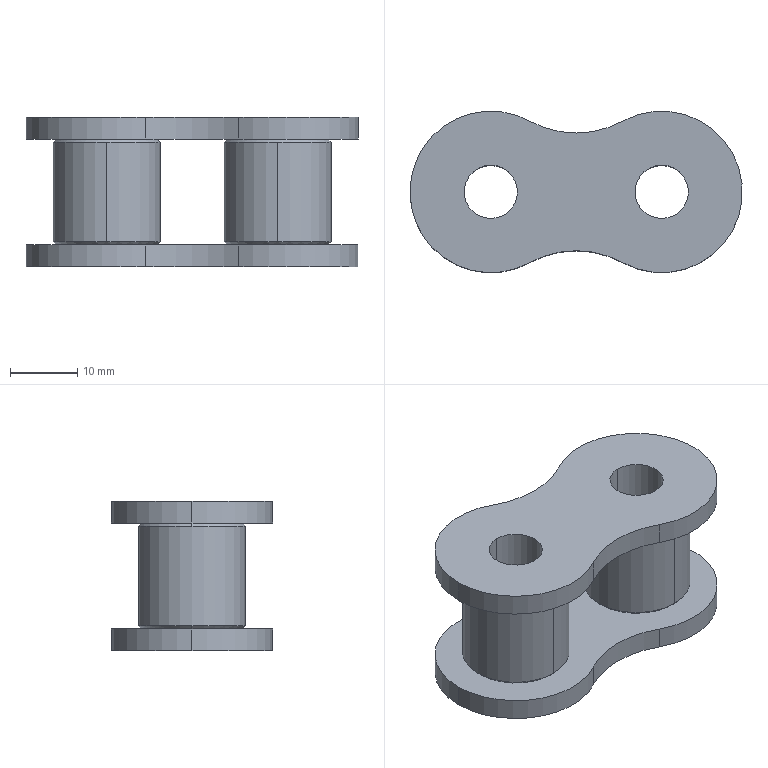Part | STEP file | chain_16a inner link | 1 solid | 30 faces | box 49.4 x 24 x 22.25 mm | volume 10373 mm3 | cylinder 18 | cone 8 | plane 4 | commonest cylinder face diameters 24 x6 7.92 x4 15.88 x4 28.8 x4